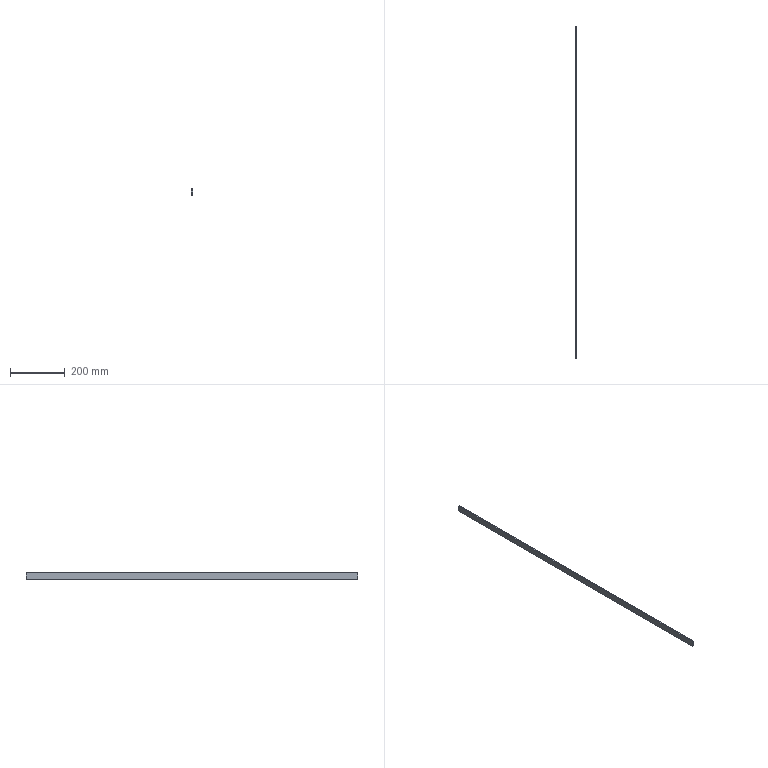Part | NX | features BREP 1 | 1 solid | 6 faces | box 4 x 1214 x 21.997 mm | volume 106850 mm3 | plane 6
STEP:
#1=CARTESIAN_POINT('',(589.385,607.17,381.004));
#2=VERTEX_POINT('',#1);
#3=CARTESIAN_POINT('',(593.385,607.17,381.004));
#4=VERTEX_POINT('',#3);
#5=CARTESIAN_POINT('',(591.385,607.17,381.004));
#6=DIRECTION('',(1.,0.,0.));
#7=VECTOR('',#6,1000.);
#8=LINE('',#5,#7);
#9=EDGE_CURVE('',#2,#4,#8,.T.);
#10=ORIENTED_EDGE('',*,*,#9,.T.);
#11=CARTESIAN_POINT('',(593.385,-607.17,381.004));
#12=VERTEX_POINT('',#11);
#13=CARTESIAN_POINT('',(593.385,0.,381.004));
#14=DIRECTION('',(0.,-1.,0.));
#15=VECTOR('',#14,1000.);
#16=LINE('',#13,#15);
#17=EDGE_CURVE('',#4,#12,#16,.T.);
#18=ORIENTED_EDGE('',*,*,#17,.T.);
#19=CARTESIAN_POINT('',(589.385,-607.17,381.004));
#20=VERTEX_POINT('',#19);
#21=CARTESIAN_POINT('',(591.385,-607.17,381.004));
#22=DIRECTION('',(1.,0.,0.));
#23=VECTOR('',#22,1000.);
#24=LINE('',#21,#23);
#25=EDGE_CURVE('',#20,#12,#24,.T.);
#26=ORIENTED_EDGE('',*,*,#25,.F.);
#27=CARTESIAN_POINT('',(589.385,0.,381.004));
#28=DIRECTION('',(0.,-1.,0.));
#29=VECTOR('',#28,1000.);
#30=LINE('',#27,#29);
#31=EDGE_CURVE('',#2,#20,#30,.T.);
#32=ORIENTED_EDGE('',*,*,#31,.F.);
#33=EDGE_LOOP('',(#10,#18,#26,#32));
#34=FACE_BOUND('',#33,.T.);
#35=CARTESIAN_POINT('',(579.388,0.001,381.004));
#36=DIRECTION('',(0.,0.,1.));
#37=DIRECTION('',(0.,-1.,0.));
#38=AXIS2_PLACEMENT_3D('',#35,#36,#37);
#39=PLANE('',#38);
#40=ADVANCED_FACE('',(#34),#39,.F.);
#41=CARTESIAN_POINT('',(593.385,607.17,403.001));
#42=VERTEX_POINT('',#41);
#43=CARTESIAN_POINT('',(593.385,607.17,392.002));
#44=DIRECTION('',(0.000000043,0.,-1.));
#45=VECTOR('',#44,1000.);
#46=LINE('',#43,#45);
#47=EDGE_CURVE('',#42,#4,#46,.T.);
#48=ORIENTED_EDGE('',*,*,#47,.T.);
#49=ORIENTED_EDGE('',*,*,#9,.F.);
#50=CARTESIAN_POINT('',(589.385,607.17,403.001));
#51=VERTEX_POINT('',#50);
#52=CARTESIAN_POINT('',(589.385,607.17,392.002));
#53=DIRECTION('',(0.000000043,0.,-1.));
#54=VECTOR('',#53,1000.);
#55=LINE('',#52,#54);
#56=EDGE_CURVE('',#51,#2,#55,.T.);
#57=ORIENTED_EDGE('',*,*,#56,.F.);
#58=CARTESIAN_POINT('',(591.385,607.17,403.001));
#59=DIRECTION('',(1.,0.,0.000000043));
#60=VECTOR('',#59,1000.);
#61=LINE('',#58,#60);
#62=EDGE_CURVE('',#51,#42,#61,.T.);
#63=ORIENTED_EDGE('',*,*,#62,.T.);
#64=EDGE_LOOP('',(#48,#49,#57,#63));
#65=FACE_BOUND('',#64,.T.);
#66=CARTESIAN_POINT('',(589.385,607.17,403.001));
#67=DIRECTION('',(0.,1.,0.));
#68=DIRECTION('',(1.,0.,0.000000043));
#69=AXIS2_PLACEMENT_3D('',#66,#67,#68);
#70=PLANE('',#69);
#71=ADVANCED_FACE('',(#65),#70,.T.);
#72=CARTESIAN_POINT('',(593.385,-607.17,403.001));
#73=VERTEX_POINT('',#72);
#74=CARTESIAN_POINT('',(593.385,0.,403.001));
#75=DIRECTION('',(0.,1.,0.));
#76=VECTOR('',#75,1000.);
#77=LINE('',#74,#76);
#78=EDGE_CURVE('',#73,#42,#77,.T.);
#79=ORIENTED_EDGE('',*,*,#78,.F.);
#80=CARTESIAN_POINT('',(593.385,-607.17,392.002));
#81=DIRECTION('',(0.000000043,0.,-1.));
#82=VECTOR('',#81,1000.);
#83=LINE('',#80,#82);
#84=EDGE_CURVE('',#73,#12,#83,.T.);
#85=ORIENTED_EDGE('',*,*,#84,.T.);
#86=ORIENTED_EDGE('',*,*,#17,.F.);
#87=ORIENTED_EDGE('',*,*,#47,.F.);
#88=EDGE_LOOP('',(#79,#85,#86,#87));
#89=FACE_BOUND('',#88,.T.);
#90=CARTESIAN_POINT('',(593.385,588.,390.501));
#91=DIRECTION('',(-1.,0.,-0.000000043));
#92=DIRECTION('',(-0.000000043,0.000003687,1.));
#93=AXIS2_PLACEMENT_3D('',#90,#91,#92);
#94=PLANE('',#93);
#95=ADVANCED_FACE('',(#89),#94,.F.);
#96=CARTESIAN_POINT('',(589.385,-607.17,403.001));
#97=VERTEX_POINT('',#96);
#98=CARTESIAN_POINT('',(591.385,-607.17,403.001));
#99=DIRECTION('',(1.,0.,0.000000043));
#100=VECTOR('',#99,1000.);
#101=LINE('',#98,#100);
#102=EDGE_CURVE('',#97,#73,#101,.T.);
#103=ORIENTED_EDGE('',*,*,#102,.F.);
#104=CARTESIAN_POINT('',(589.385,-607.17,392.002));
#105=DIRECTION('',(0.000000043,0.,-1.));
#106=VECTOR('',#105,1000.);
#107=LINE('',#104,#106);
#108=EDGE_CURVE('',#97,#20,#107,.T.);
#109=ORIENTED_EDGE('',*,*,#108,.T.);
#110=ORIENTED_EDGE('',*,*,#25,.T.);
#111=ORIENTED_EDGE('',*,*,#84,.F.);
#112=EDGE_LOOP('',(#103,#109,#110,#111));
#113=FACE_BOUND('',#112,.T.);
#114=CARTESIAN_POINT('',(589.385,-607.17,403.001));
#115=DIRECTION('',(0.,1.,0.));
#116=DIRECTION('',(1.,0.,0.000000043));
#117=AXIS2_PLACEMENT_3D('',#114,#115,#116);
#118=PLANE('',#117);
#119=ADVANCED_FACE('',(#113),#118,.F.);
#120=ORIENTED_EDGE('',*,*,#56,.T.);
#121=ORIENTED_EDGE('',*,*,#31,.T.);
#122=ORIENTED_EDGE('',*,*,#108,.F.);
#123=CARTESIAN_POINT('',(589.385,0.,403.001));
#124=DIRECTION('',(0.,1.,0.));
#125=VECTOR('',#124,1000.);
#126=LINE('',#123,#125);
#127=EDGE_CURVE('',#97,#51,#126,.T.);
#128=ORIENTED_EDGE('',*,*,#127,.T.);
#129=EDGE_LOOP('',(#120,#121,#122,#128));
#130=FACE_BOUND('',#129,.T.);
#131=CARTESIAN_POINT('',(589.385,588.,390.501));
#132=DIRECTION('',(-1.,0.,-0.000000043));
#133=DIRECTION('',(-0.000000043,0.000003687,1.));
#134=AXIS2_PLACEMENT_3D('',#131,#132,#133);
#135=PLANE('',#134);
#136=ADVANCED_FACE('',(#130),#135,.T.);
#137=ORIENTED_EDGE('',*,*,#127,.F.);
#138=ORIENTED_EDGE('',*,*,#102,.T.);
#139=ORIENTED_EDGE('',*,*,#78,.T.);
#140=ORIENTED_EDGE('',*,*,#62,.F.);
#141=EDGE_LOOP('',(#137,#138,#139,#140));
#142=FACE_BOUND('',#141,.T.);
#143=CARTESIAN_POINT('',(591.385,588.,403.001));
#144=DIRECTION('',(0.000000043,0.,-1.));
#145=DIRECTION('',(1.,0.,0.000000043));
#146=AXIS2_PLACEMENT_3D('',#143,#144,#145);
#147=PLANE('',#146);
#148=ADVANCED_FACE('',(#142),#147,.F.);
#149=CLOSED_SHELL('',(#40,#71,#95,#119,#136,#148));
#150=MANIFOLD_SOLID_BREP('',#149);
#151=(LENGTH_UNIT()NAMED_UNIT(*)SI_UNIT(.MILLI.,.METRE.));
#152=UNCERTAINTY_MEASURE_WITH_UNIT(LENGTH_MEASURE(0.00001),#151,'','');
#153=(NAMED_UNIT(*)PLANE_ANGLE_UNIT()SI_UNIT($,.RADIAN.));
#154=(NAMED_UNIT(*)SI_UNIT($,.STERADIAN.)SOLID_ANGLE_UNIT());
#155=(GEOMETRIC_REPRESENTATION_CONTEXT(3)GLOBAL_UNCERTAINTY_ASSIGNED_CONTEXT((#152))GLOBAL_UNIT_ASSIGNED_CONTEXT((#151,#153,#154))REPRESENTATION_CONTEXT('',''));
#156=ADVANCED_BREP_SHAPE_REPRESENTATION('',(#150),#155);